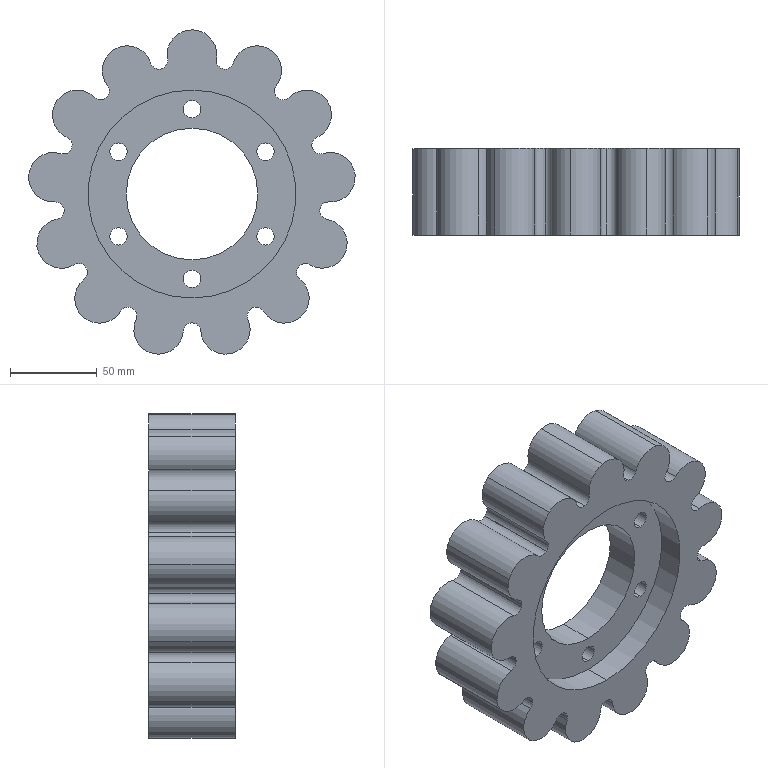Part | SolidWorks | features ICE 2, CirPattern 1, Extrusion 1 | 1 solid | 100 faces | box 188.466 x 50 x 187.3 mm | volume 763094 mm3 | cylinder 96 | plane 4 | commonest cylinder face diameters 10 x38 28.613 x26 148.78 x13 158.465 x13 120 x4 76 x2